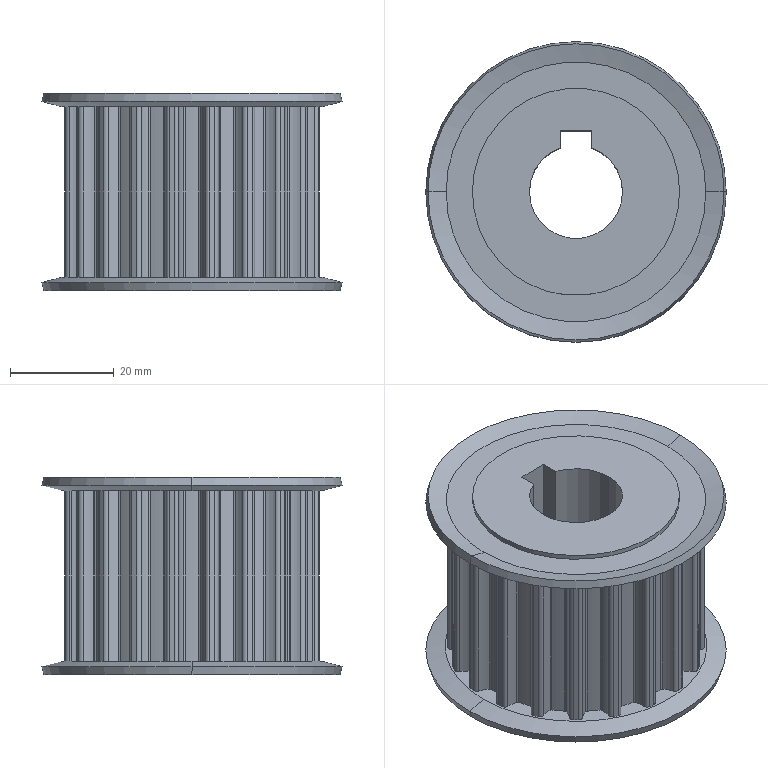Part | SolidWorks | features BaseBody 1, ICE 1 | 1 solid | 209 faces | box 58 x 58 x 38.085 mm | volume 55625 mm3 | cylinder 188 | cone 12 | plane 9 | commonest cylinder face diameters 1.5 x50 0.8 x46 10.6 x44 43.9 x21 49.56 x20 40 x4